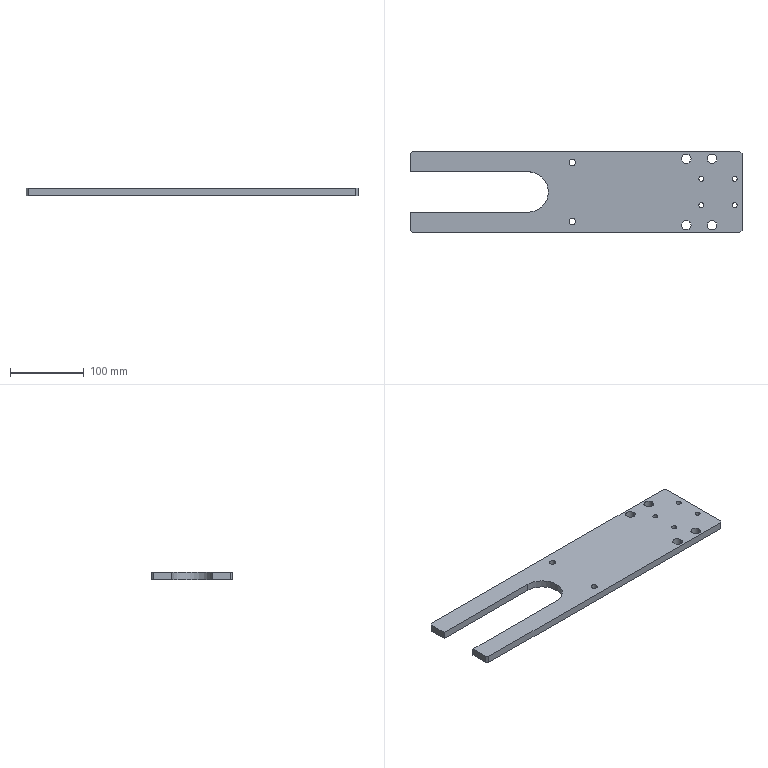Part | STEP file | Adjusting plate XG | 1 solid | 34 faces | box 450 x 110 x 10 mm | volume 387044 mm3 | cylinder 21 | plane 13 | commonest cylinder face diameters 6.8 x8 13 x8 8.5 x4 55 x1